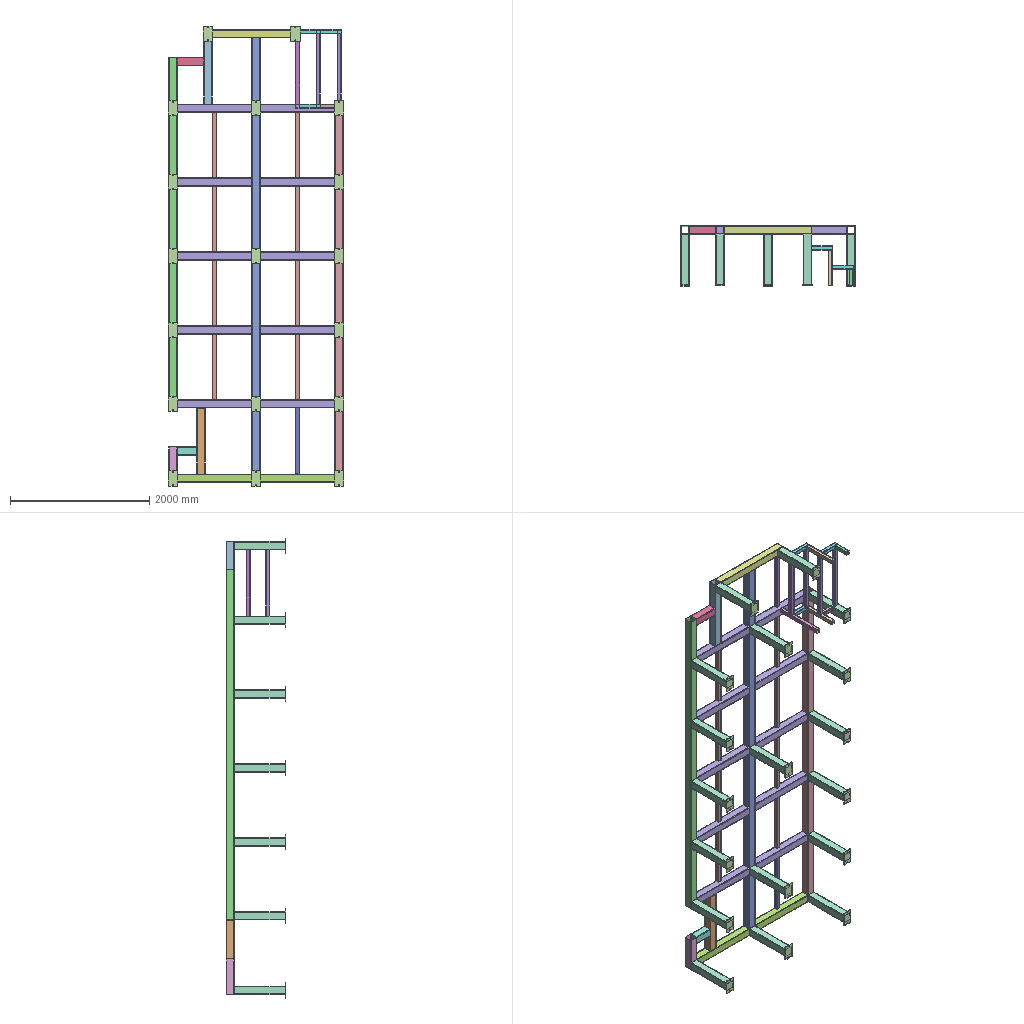Assembly | SolidWorks | 22 different items | 78 placed | box 2520 x 860 x 6600 mm
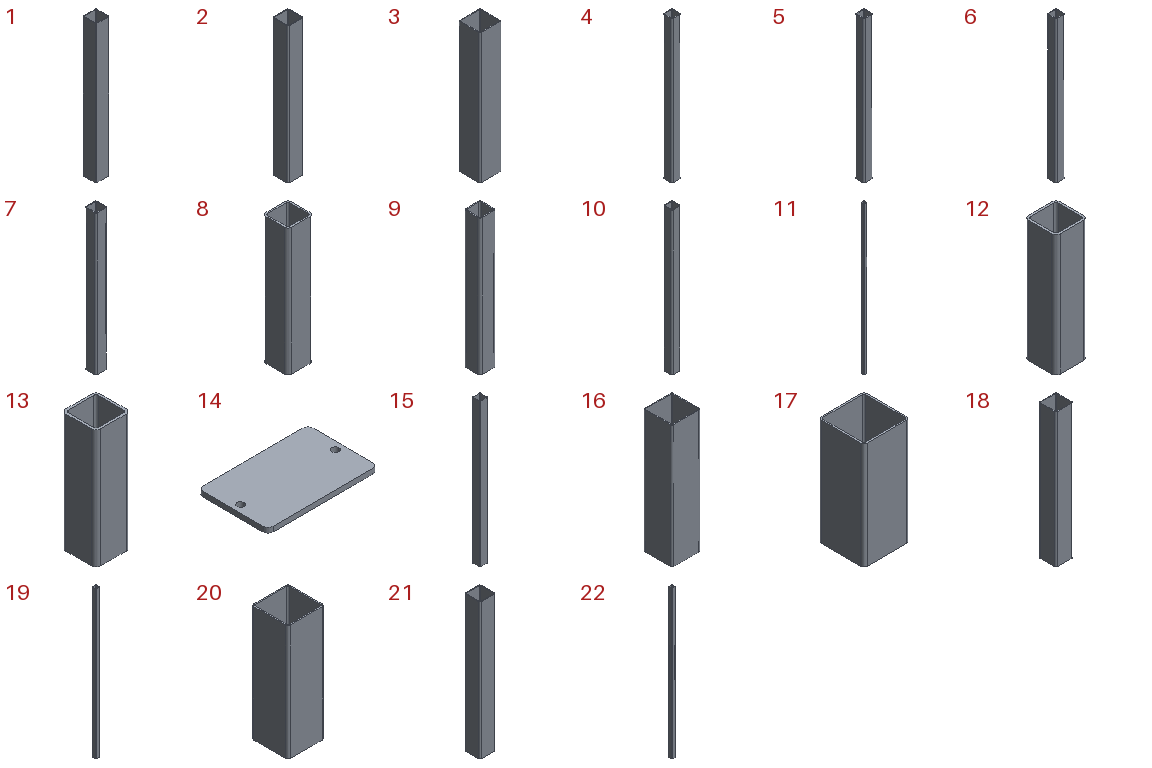Parts list (item | quantity | size | volume | features):
1 | x1 | 120 x 120 x 1255 mm | 2277570 mm3 | features ICE 1, LibraryFeature 1
2 | x10 | 120 x 120 x 1070 mm | 1941832 mm3 | features ICE 1, LibraryFeature 1
3 | x18 | 120 x 120 x 730 mm | 1324801 mm3 | features ICE 1, LibraryFeature 1
4 | x8 | 60 x 60 x 940 mm | 803509 mm3 | features ICE 1, LibraryFeature 1
5 | x2 | 60 x 60 x 950 mm | 812057 mm3 | features ICE 1, LibraryFeature 1
6 | x1 | 60 x 60 x 945 mm | 807783 mm3 | features ICE 1, LibraryFeature 1
7 | x1 | 60 x 60 x 740 mm | 632549 mm3 | features ICE 1, LibraryFeature 1
8 | x3 | 60 x 60 x 300 mm | 256439 mm3 | features ICE 1, LibraryFeature 1
9 | x2 | 60 x 60 x 510 mm | 435946 mm3 | features ICE 1, LibraryFeature 1
10 | x3 | 60 x 60 x 1010 mm | 863344 mm3 | features ICE 1, LibraryFeature 1
11 | x1 | 120 x 120 x 6260 mm | 11360626 mm3 | features ICE 1, LibraryFeature 1
12 | x1 | 60 x 60 x 230 mm | 196603 mm3 | features ICE 1, LibraryFeature 1
13 | x1 | 60 x 60 x 205 mm | 175233 mm3 | features ICE 1, LibraryFeature 1
14 | x18 | 220 x 140 x 10 mm | 304063 mm3 | features Extrusion 1, Fillet 1
15 | x1 | 120 x 120 x 2260 mm | 4101440 mm3 | features ICE 1, LibraryFeature 1
16 | x1 | 120 x 120 x 510 mm | 925546 mm3 | features ICE 1, LibraryFeature 1
17 | x1 | 120 x 120 x 280 mm | 508143 mm3 | features ICE 1, LibraryFeature 1
18 | x1 | 120 x 120 x 945 mm | 1714983 mm3 | features ICE 1, LibraryFeature 1
19 | x1 | 120 x 120 x 5030 mm | 9128426 mm3 | features ICE 1, LibraryFeature 1
20 | x1 | 120 x 120 x 380 mm | 689623 mm3 | features ICE 1, LibraryFeature 1
21 | x1 | 120 x 120 x 1070 mm | 1941832 mm3 | features ICE 1, LibraryFeature 1
22 | x1 | 120 x 120 x 5430 mm | 9854345 mm3 | features ICE 1, LibraryFeature 1
Mates (type | each side: item.copy, entity, surface, feature):
Coincident | 22.1 face plane Boss-Extrude1 | 11.1 face plane Boss-Extrude1
Coincident | 22.1 face plane Boss-Extrude1 | 15.1 face plane Boss-Extrude1 | 3 times
Coincident | 11.1 face plane Boss-Extrude1 | 15.1 face plane Boss-Extrude1
Coincident | 15.1 face plane Boss-Extrude1 | 16.1 face plane Boss-Extrude1 | 3 times
Width | 11.1 face plane Boss-Extrude1 | 11.1 face plane Boss-Extrude1 | 16.1 face plane Boss-Extrude1 | 22.1 face plane Boss-Extrude1
Coincident | 16.1 face plane Boss-Extrude1 | 17.1 face plane Boss-Extrude1 | 3 times
Coincident | 17.1 face plane Boss-Extrude1 | 18.1 face plane Boss-Extrude1 | 2 times
Coincident | 18.1 face plane Boss-Extrude1 | 2.1 face plane Boss-Extrude1
Coincident | 2.1 face plane Boss-Extrude1 | 19.1 face plane Boss-Extrude1 | 3 times
Coincident | 19.1 face plane Boss-Extrude1 | 20.1 face plane Boss-Extrude1 | 3 times
Coincident | 20.1 face plane Boss-Extrude1 | 21.1 face plane Boss-Extrude1 | 2 times
Coincident | 21.1 face plane Boss-Extrude1 | 1.1 face plane Boss-Extrude1 | 3 times
Coincident | 19.1 face plane Boss-Extrude1 | 2.2 face plane Boss-Extrude1
Coincident | 11.1 face plane Boss-Extrude1 | 2.2 face plane Boss-Extrude1
DistanceDim | 2.2 face plane Boss-Extrude1 | 2.1 face plane Boss-Extrude1
Coincident | 22.1 face plane Boss-Extrude1 | 2.3 face plane Boss-Extrude1 | 2 times
Coincident | 2.2 face plane Boss-Extrude1 | 2.3 face plane Boss-Extrude1
Coincident | 19.1 face plane Boss-Extrude1 | 2.4 face plane Boss-Extrude1
Coincident | 2.2 face plane Boss-Extrude1 | 2.4 face plane Boss-Extrude1
DistanceDim | 2.4 face plane Boss-Extrude1 | 2.2 face plane Boss-Extrude1
Coincident | 11.1 face plane Boss-Extrude1 | 2.5 face plane Boss-Extrude1
Coincident | 2.4 face plane Boss-Extrude1 | 2.5 face plane Boss-Extrude1 | 2 times
Coincident | 19.1 face plane Boss-Extrude1 | 2.6 face plane Boss-Extrude1
Coincident | 2.4 face plane Boss-Extrude1 | 2.6 face plane Boss-Extrude1
DistanceDim | 2.6 face plane Boss-Extrude1 | 2.4 face plane Boss-Extrude1
Coincident | 22.1 face plane Boss-Extrude1 | 2.7 face plane Boss-Extrude1
Coincident | 2.6 face plane Boss-Extrude1 | 2.7 face plane Boss-Extrude1 | 2 times
Coincident | 1.1 face plane Boss-Extrude1 | 5.1 face plane Boss-Extrude1 | 3 times
Coincident | 11.1 face plane Boss-Extrude1 | 1.1 face plane Boss-Extrude1
Coincident | 15.1 face plane Boss-Extrude1 | 18.1 face plane Boss-Extrude1
Coincident | 16.1 face plane Boss-Extrude1 | 3.1 face plane Boss-Extrude1 | 2 times
Coincident | 15.1 face plane Boss-Extrude1 | 3.1 face plane Boss-Extrude1
Coincident | 15.1 face plane Boss-Extrude1 | 3.2 face plane Boss-Extrude1 | 2 times
Coincident | 11.1 face plane Boss-Extrude1 | 3.2 face plane Boss-Extrude1
Coincident | 22.1 face plane Boss-Extrude1 | 3.3 face plane Boss-Extrude1 | 2 times
Coincident | 15.1 face plane Boss-Extrude1 | 3.3 face plane Boss-Extrude1
Coincident | 19.1 face plane Boss-Extrude1 | 3.4 face plane Boss-Extrude1 | 2 times
Coincident | 2.2 face plane Boss-Extrude1 | 3.4 face plane Boss-Extrude1
Coincident | 11.1 face plane Boss-Extrude1 | 3.5 face plane Boss-Extrude1 | 2 times
Coincident | 22.1 face plane Boss-Extrude1 | 3.6 face plane Boss-Extrude1 | 2 times
Coincident | 2.3 face plane Boss-Extrude1 | 3.6 face plane Boss-Extrude1
Coincident | 22.1 face plane Boss-Extrude1 | 3.7 face plane Boss-Extrude1 | 2 times
Coincident | 2.5 face plane Boss-Extrude1 | 3.7 face plane Boss-Extrude1
Coincident | 11.1 face plane Boss-Extrude1 | 3.8 face plane Boss-Extrude1 | 2 times
Coincident | 19.1 face plane Boss-Extrude1 | 3.9 face plane Boss-Extrude1 | 2 times
Coincident | 2.4 face plane Boss-Extrude1 | 3.9 face plane Boss-Extrude1
Coincident | 22.1 face plane Boss-Extrude1 | 3.10 face plane Boss-Extrude1 | 2 times
Coincident | 2.7 face plane Boss-Extrude1 | 3.10 face plane Boss-Extrude1
Coincident | 11.1 face plane Boss-Extrude1 | 3.11 face plane Boss-Extrude1 | 2 times
Coincident | 19.1 face plane Boss-Extrude1 | 3.12 face plane Boss-Extrude1 | 2 times
Coincident | 2.6 face plane Boss-Extrude1 | 3.12 face plane Boss-Extrude1
Coincident | 22.1 face plane Boss-Extrude1 | 3.13 face plane Boss-Extrude1 | 3 times
Coincident | 1.1 face plane Boss-Extrude1 | 3.14 face plane Boss-Extrude1 | 3 times
Coincident | 21.1 face plane Boss-Extrude1 | 3.15 face plane Boss-Extrude1 | 2 times
Coincident | 1.1 face plane Boss-Extrude1 | 3.15 face plane Boss-Extrude1
Coincident | 11.1 face plane Boss-Extrude1 | 2.8 face plane Boss-Extrude1
Coincident | 22.1 face plane Boss-Extrude1 | 2.8 face plane Boss-Extrude1 | 2 times
Coincident | 19.1 face plane Boss-Extrude1 | 2.9 face plane Boss-Extrude1
Coincident | 2.8 face plane Boss-Extrude1 | 2.9 face plane Boss-Extrude1 | 2 times
Coincident | 19.1 face plane Boss-Extrude1 | 3.16 face plane Boss-Extrude1 | 2 times
Coincident | 2.9 face plane Boss-Extrude1 | 3.16 face plane Boss-Extrude1
Coincident | 3.8 face plane Boss-Extrude1 | 2.8 face plane Boss-Extrude1
Coincident | 2.9 face plane Boss-Extrude1 | 4.1 face plane Boss-Extrude1 | 2 times
Width | 4.1 face plane Boss-Extrude1 | 4.1 face plane Boss-Extrude1 | 19.1 face plane Boss-Extrude1 | 11.1 face plane Boss-Extrude1
Coincident | 2.8 face plane Boss-Extrude1 | 4.2 face plane Boss-Extrude1
Coincident | 4.1 face plane Boss-Extrude1 | 4.2 face plane Boss-Extrude1
Width | 4.2 face plane Boss-Extrude1 | 4.2 face plane Boss-Extrude1 | 11.1 face plane Boss-Extrude1 | 22.1 face plane Boss-Extrude1
Coincident | 3.3 face plane Boss-Extrude1 | 14.1 face plane Boss-Extrude1
Width | 14.1 face plane Boss-Extrude1 | 14.1 face plane Boss-Extrude1 | 3.3 face plane Boss-Extrude1 | 3.3 face plane Boss-Extrude1 | 2 times
Coincident | 2.8 face plane Boss-Extrude1 | 7.1 face plane Boss-Extrude1 | 2 times
Coincident | 5.1 face plane Boss-Extrude1 | 7.1 face plane Boss-Extrude1
Coincident | 7.1 face plane Boss-Extrude1 | 5.2 face plane Boss-Extrude1
Coincident | 3.14 face plane Boss-Extrude1 | 5.2 face plane Boss-Extrude1
DistanceDim | 5.2 face plane Boss-Extrude1 | 5.1 face plane Boss-Extrude1
Coincident | 3.14 face plane Boss-Extrude1 | 8.1 face plane Boss-Extrude1 | 2 times
Coincident | 5.2 face plane Boss-Extrude1 | 8.1 face plane Boss-Extrude1
Coincident | 7.1 face plane Boss-Extrude1 | 8.2 face plane Boss-Extrude1 | 2 times
Coincident | 5.2 face plane Boss-Extrude1 | 8.2 face plane Boss-Extrude1
Coincident | 8.1 face plane Boss-Extrude1 | 9.1 face plane Boss-Extrude1 | 3 times
Coincident | 8.2 face plane Boss-Extrude1 | 9.2 face plane Boss-Extrude1 | 3 times
Coincident | 8.1 face plane Boss-Extrude1 | 10.1 face plane Boss-Extrude1 | 2 times
Coincident | 9.1 face plane Boss-Extrude1 | 10.1 face plane Boss-Extrude1
Coincident | 9.1 face plane Boss-Extrude1 | 8.3 face plane Boss-Extrude1 | 2 times
DistanceDim | 8.1 face plane Boss-Extrude1 | 8.3 face plane Boss-Extrude1
Coincident | 8.3 face plane Boss-Extrude1 | 12.1 face plane Boss-Extrude1 | 3 times
Coincident | 8.3 face plane Boss-Extrude1 | 10.2 face plane Boss-Extrude1 | 2 times
Coincident | 12.1 face plane Boss-Extrude1 | 10.2 face plane Boss-Extrude1
Coincident | 9.2 face plane Boss-Extrude1 | 13.1 face plane Boss-Extrude1 | 2 times
Coincident | 8.3 face plane Boss-Extrude1 | 13.1 face plane Boss-Extrude1
Coincident | 9.1 face plane Boss-Extrude1 | 10.3 face plane Boss-Extrude1 | 2 times
Coincident | 8.3 face plane Boss-Extrude1 | 10.3 face plane Boss-Extrude1
Coincident | 11.1 face plane Boss-Extrude1 | 2.1 face plane Boss-Extrude1
Coincident | 11.1 face plane Boss-Extrude1 | 2.10 face plane Boss-Extrude1
Coincident | 2.1 face plane Boss-Extrude1 | 2.10 face plane Boss-Extrude1 | 2 times
DistanceDim | 2.1 face plane Boss-Extrude1 | 15.1 face plane Boss-Extrude1
Coincident | 6.1 face plane Boss-Extrude1 | 2.10 face plane Boss-Extrude1 | 2 times
Coincident | 4.2 face plane Boss-Extrude1 | 6.1 face plane Boss-Extrude1
Coincident | 2.4 face plane Boss-Extrude1 | 3.11 face plane Boss-Extrude1
Coincident | 2.1 face plane Boss-Extrude1 | 3.5 face plane Boss-Extrude1
Coincident | 22.1 face plane Boss-Extrude1 | 3.17 face plane Boss-Extrude1 | 2 times
Coincident | 2.10 face plane Boss-Extrude1 | 3.17 face plane Boss-Extrude1
Coincident | 19.1 face plane Boss-Extrude1 | 3.18 face plane Boss-Extrude1 | 2 times
Coincident | 2.1 face plane Boss-Extrude1 | 3.18 face plane Boss-Extrude1